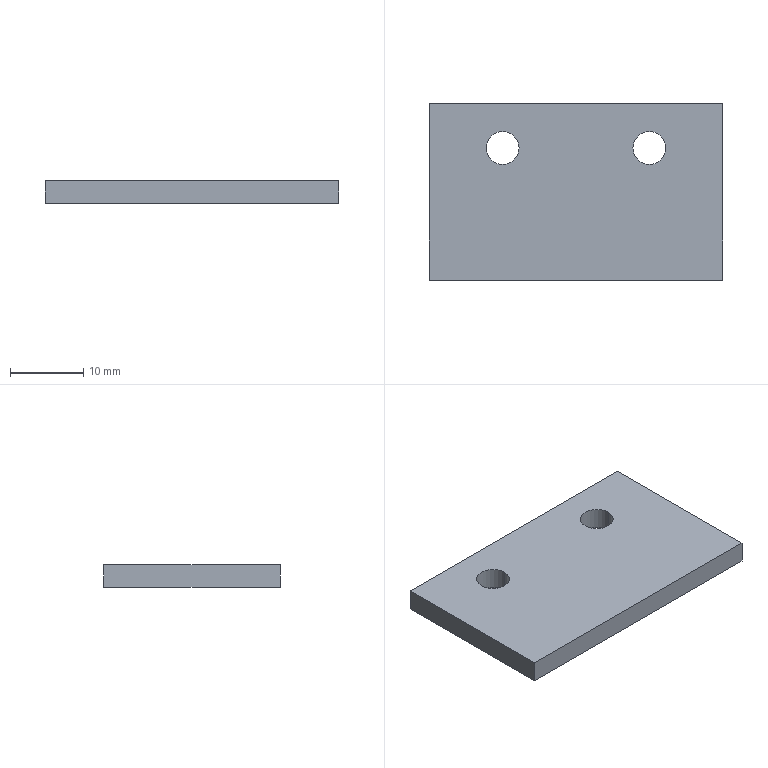Part | STEP file | Guide pressure plate | 1 solid | 10 faces | box 40 x 24 x 3 mm | volume 2785 mm3 | plane 6 | cylinder 4 | commonest cylinder face diameters 4.5 x4
STEP:
#1=CARTESIAN_POINT('',(7.75,6.,0.));
#2=VERTEX_POINT('',#1);
#3=CARTESIAN_POINT('',(12.25,6.,0.));
#4=VERTEX_POINT('',#3);
#5=CARTESIAN_POINT('',(10.,6.,0.));
#6=DIRECTION('',(0.,0.,1.));
#7=DIRECTION('',(1.,0.,0.));
#8=AXIS2_PLACEMENT_3D('',#5,#6,#7);
#9=CIRCLE('',#8,2.25);
#10=EDGE_CURVE('',#2,#4,#9,.T.);
#11=ORIENTED_EDGE('',*,*,#10,.F.);
#12=CARTESIAN_POINT('',(7.75,6.,3.));
#13=VERTEX_POINT('',#12);
#14=CARTESIAN_POINT('',(7.75,6.,0.));
#15=DIRECTION('',(0.,0.,1.));
#16=VECTOR('',#15,1000.);
#17=LINE('',#14,#16);
#18=EDGE_CURVE('',#2,#13,#17,.T.);
#19=ORIENTED_EDGE('',*,*,#18,.T.);
#20=CARTESIAN_POINT('',(12.25,6.,3.));
#21=VERTEX_POINT('',#20);
#22=CARTESIAN_POINT('',(10.,6.,3.));
#23=DIRECTION('',(0.,0.,1.));
#24=DIRECTION('',(1.,0.,0.));
#25=AXIS2_PLACEMENT_3D('',#22,#23,#24);
#26=CIRCLE('',#25,2.25);
#27=EDGE_CURVE('',#13,#21,#26,.T.);
#28=ORIENTED_EDGE('',*,*,#27,.T.);
#29=CARTESIAN_POINT('',(12.25,6.,0.));
#30=DIRECTION('',(0.,0.,1.));
#31=VECTOR('',#30,1000.);
#32=LINE('',#29,#31);
#33=EDGE_CURVE('',#4,#21,#32,.T.);
#34=ORIENTED_EDGE('',*,*,#33,.F.);
#35=EDGE_LOOP('',(#11,#19,#28,#34));
#36=FACE_OUTER_BOUND('',#35,.T.);
#37=CARTESIAN_POINT('',(10.,6.,0.));
#38=DIRECTION('',(0.,0.,1.));
#39=DIRECTION('',(1.,0.,0.));
#40=AXIS2_PLACEMENT_3D('',#37,#38,#39);
#41=CYLINDRICAL_SURFACE('',#40,2.25);
#42=ADVANCED_FACE('',(#36),#41,.F.);
#43=CARTESIAN_POINT('',(-12.25,6.,0.));
#44=VERTEX_POINT('',#43);
#45=CARTESIAN_POINT('',(-7.75,6.,0.));
#46=VERTEX_POINT('',#45);
#47=CARTESIAN_POINT('',(-10.,6.,0.));
#48=DIRECTION('',(0.,0.,1.));
#49=DIRECTION('',(1.,0.,0.));
#50=AXIS2_PLACEMENT_3D('',#47,#48,#49);
#51=CIRCLE('',#50,2.25);
#52=EDGE_CURVE('',#44,#46,#51,.T.);
#53=ORIENTED_EDGE('',*,*,#52,.F.);
#54=CARTESIAN_POINT('',(-12.25,6.,3.));
#55=VERTEX_POINT('',#54);
#56=CARTESIAN_POINT('',(-12.25,6.,0.));
#57=DIRECTION('',(0.,0.,1.));
#58=VECTOR('',#57,1000.);
#59=LINE('',#56,#58);
#60=EDGE_CURVE('',#44,#55,#59,.T.);
#61=ORIENTED_EDGE('',*,*,#60,.T.);
#62=CARTESIAN_POINT('',(-7.75,6.,3.));
#63=VERTEX_POINT('',#62);
#64=CARTESIAN_POINT('',(-10.,6.,3.));
#65=DIRECTION('',(0.,0.,1.));
#66=DIRECTION('',(1.,0.,0.));
#67=AXIS2_PLACEMENT_3D('',#64,#65,#66);
#68=CIRCLE('',#67,2.25);
#69=EDGE_CURVE('',#55,#63,#68,.T.);
#70=ORIENTED_EDGE('',*,*,#69,.T.);
#71=CARTESIAN_POINT('',(-7.75,6.,0.));
#72=DIRECTION('',(0.,0.,1.));
#73=VECTOR('',#72,1000.);
#74=LINE('',#71,#73);
#75=EDGE_CURVE('',#46,#63,#74,.T.);
#76=ORIENTED_EDGE('',*,*,#75,.F.);
#77=EDGE_LOOP('',(#53,#61,#70,#76));
#78=FACE_OUTER_BOUND('',#77,.T.);
#79=CARTESIAN_POINT('',(-10.,6.,0.));
#80=DIRECTION('',(0.,0.,1.));
#81=DIRECTION('',(1.,0.,0.));
#82=AXIS2_PLACEMENT_3D('',#79,#80,#81);
#83=CYLINDRICAL_SURFACE('',#82,2.25);
#84=ADVANCED_FACE('',(#78),#83,.F.);
#85=CARTESIAN_POINT('',(20.,-12.,0.));
#86=VERTEX_POINT('',#85);
#87=CARTESIAN_POINT('',(20.,12.,0.));
#88=VERTEX_POINT('',#87);
#89=CARTESIAN_POINT('',(20.,12.,0.));
#90=DIRECTION('',(0.,1.,0.));
#91=VECTOR('',#90,1000.);
#92=LINE('',#89,#91);
#93=EDGE_CURVE('',#86,#88,#92,.T.);
#94=ORIENTED_EDGE('',*,*,#93,.T.);
#95=CARTESIAN_POINT('',(20.,12.,3.));
#96=VERTEX_POINT('',#95);
#97=CARTESIAN_POINT('',(20.,12.,3.));
#98=DIRECTION('',(0.,0.,-1.));
#99=VECTOR('',#98,1000.);
#100=LINE('',#97,#99);
#101=EDGE_CURVE('',#96,#88,#100,.T.);
#102=ORIENTED_EDGE('',*,*,#101,.F.);
#103=CARTESIAN_POINT('',(20.,-12.,3.));
#104=VERTEX_POINT('',#103);
#105=CARTESIAN_POINT('',(20.,12.,3.));
#106=DIRECTION('',(0.,1.,0.));
#107=VECTOR('',#106,1000.);
#108=LINE('',#105,#107);
#109=EDGE_CURVE('',#104,#96,#108,.T.);
#110=ORIENTED_EDGE('',*,*,#109,.F.);
#111=CARTESIAN_POINT('',(20.,-12.,3.));
#112=DIRECTION('',(0.,0.,-1.));
#113=VECTOR('',#112,1000.);
#114=LINE('',#111,#113);
#115=EDGE_CURVE('',#104,#86,#114,.T.);
#116=ORIENTED_EDGE('',*,*,#115,.T.);
#117=EDGE_LOOP('',(#94,#102,#110,#116));
#118=FACE_OUTER_BOUND('',#117,.T.);
#119=CARTESIAN_POINT('',(20.,12.,3.));
#120=DIRECTION('',(-1.,0.,0.));
#121=DIRECTION('',(0.,-1.,0.));
#122=AXIS2_PLACEMENT_3D('',#119,#120,#121);
#123=PLANE('',#122);
#124=ADVANCED_FACE('',(#118),#123,.F.);
#125=CARTESIAN_POINT('',(-20.,12.,0.));
#126=VERTEX_POINT('',#125);
#127=CARTESIAN_POINT('',(-20.,12.,0.));
#128=DIRECTION('',(-1.,0.,0.));
#129=VECTOR('',#128,1000.);
#130=LINE('',#127,#129);
#131=EDGE_CURVE('',#88,#126,#130,.T.);
#132=ORIENTED_EDGE('',*,*,#131,.T.);
#133=CARTESIAN_POINT('',(-20.,12.,3.));
#134=VERTEX_POINT('',#133);
#135=CARTESIAN_POINT('',(-20.,12.,3.));
#136=DIRECTION('',(0.,0.,-1.));
#137=VECTOR('',#136,1000.);
#138=LINE('',#135,#137);
#139=EDGE_CURVE('',#134,#126,#138,.T.);
#140=ORIENTED_EDGE('',*,*,#139,.F.);
#141=CARTESIAN_POINT('',(-20.,12.,3.));
#142=DIRECTION('',(-1.,0.,0.));
#143=VECTOR('',#142,1000.);
#144=LINE('',#141,#143);
#145=EDGE_CURVE('',#96,#134,#144,.T.);
#146=ORIENTED_EDGE('',*,*,#145,.F.);
#147=ORIENTED_EDGE('',*,*,#101,.T.);
#148=EDGE_LOOP('',(#132,#140,#146,#147));
#149=FACE_OUTER_BOUND('',#148,.T.);
#150=CARTESIAN_POINT('',(-20.,12.,3.));
#151=DIRECTION('',(0.,-1.,0.));
#152=DIRECTION('',(0.,0.,-1.));
#153=AXIS2_PLACEMENT_3D('',#150,#151,#152);
#154=PLANE('',#153);
#155=ADVANCED_FACE('',(#149),#154,.F.);
#156=CARTESIAN_POINT('',(-20.,-12.,0.));
#157=VERTEX_POINT('',#156);
#158=CARTESIAN_POINT('',(-20.,12.,0.));
#159=DIRECTION('',(0.,-1.,0.));
#160=VECTOR('',#159,1000.);
#161=LINE('',#158,#160);
#162=EDGE_CURVE('',#126,#157,#161,.T.);
#163=ORIENTED_EDGE('',*,*,#162,.T.);
#164=CARTESIAN_POINT('',(-20.,-12.,3.));
#165=VERTEX_POINT('',#164);
#166=CARTESIAN_POINT('',(-20.,-12.,3.));
#167=DIRECTION('',(0.,0.,-1.));
#168=VECTOR('',#167,1000.);
#169=LINE('',#166,#168);
#170=EDGE_CURVE('',#165,#157,#169,.T.);
#171=ORIENTED_EDGE('',*,*,#170,.F.);
#172=CARTESIAN_POINT('',(-20.,12.,3.));
#173=DIRECTION('',(0.,-1.,0.));
#174=VECTOR('',#173,1000.);
#175=LINE('',#172,#174);
#176=EDGE_CURVE('',#134,#165,#175,.T.);
#177=ORIENTED_EDGE('',*,*,#176,.F.);
#178=ORIENTED_EDGE('',*,*,#139,.T.);
#179=EDGE_LOOP('',(#163,#171,#177,#178));
#180=FACE_OUTER_BOUND('',#179,.T.);
#181=CARTESIAN_POINT('',(-20.,12.,3.));
#182=DIRECTION('',(1.,0.,0.));
#183=DIRECTION('',(0.,1.,0.));
#184=AXIS2_PLACEMENT_3D('',#181,#182,#183);
#185=PLANE('',#184);
#186=ADVANCED_FACE('',(#180),#185,.F.);
#187=CARTESIAN_POINT('',(-20.,-12.,0.));
#188=DIRECTION('',(1.,0.,0.));
#189=VECTOR('',#188,1000.);
#190=LINE('',#187,#189);
#191=EDGE_CURVE('',#157,#86,#190,.T.);
#192=ORIENTED_EDGE('',*,*,#191,.T.);
#193=ORIENTED_EDGE('',*,*,#115,.F.);
#194=CARTESIAN_POINT('',(-20.,-12.,3.));
#195=DIRECTION('',(1.,0.,0.));
#196=VECTOR('',#195,1000.);
#197=LINE('',#194,#196);
#198=EDGE_CURVE('',#165,#104,#197,.T.);
#199=ORIENTED_EDGE('',*,*,#198,.F.);
#200=ORIENTED_EDGE('',*,*,#170,.T.);
#201=EDGE_LOOP('',(#192,#193,#199,#200));
#202=FACE_OUTER_BOUND('',#201,.T.);
#203=CARTESIAN_POINT('',(-20.,-12.,3.));
#204=DIRECTION('',(0.,1.,0.));
#205=DIRECTION('',(0.,0.,1.));
#206=AXIS2_PLACEMENT_3D('',#203,#204,#205);
#207=PLANE('',#206);
#208=ADVANCED_FACE('',(#202),#207,.F.);
#209=CARTESIAN_POINT('',(10.,6.,3.));
#210=DIRECTION('',(0.,0.,1.));
#211=DIRECTION('',(1.,0.,0.));
#212=AXIS2_PLACEMENT_3D('',#209,#210,#211);
#213=CIRCLE('',#212,2.25);
#214=EDGE_CURVE('',#21,#13,#213,.T.);
#215=ORIENTED_EDGE('',*,*,#214,.F.);
#216=ORIENTED_EDGE('',*,*,#27,.F.);
#217=EDGE_LOOP('',(#215,#216));
#218=FACE_BOUND('',#217,.T.);
#219=CARTESIAN_POINT('',(-10.,6.,3.));
#220=DIRECTION('',(0.,0.,1.));
#221=DIRECTION('',(1.,0.,0.));
#222=AXIS2_PLACEMENT_3D('',#219,#220,#221);
#223=CIRCLE('',#222,2.25);
#224=EDGE_CURVE('',#63,#55,#223,.T.);
#225=ORIENTED_EDGE('',*,*,#224,.F.);
#226=ORIENTED_EDGE('',*,*,#69,.F.);
#227=EDGE_LOOP('',(#225,#226));
#228=FACE_BOUND('',#227,.T.);
#229=ORIENTED_EDGE('',*,*,#109,.T.);
#230=ORIENTED_EDGE('',*,*,#145,.T.);
#231=ORIENTED_EDGE('',*,*,#176,.T.);
#232=ORIENTED_EDGE('',*,*,#198,.T.);
#233=EDGE_LOOP('',(#229,#230,#231,#232));
#234=FACE_OUTER_BOUND('',#233,.T.);
#235=CARTESIAN_POINT('',(0.,0.,3.));
#236=DIRECTION('',(0.,0.,1.));
#237=DIRECTION('',(1.,0.,0.));
#238=AXIS2_PLACEMENT_3D('',#235,#236,#237);
#239=PLANE('',#238);
#240=ADVANCED_FACE('',(#218,#228,#234),#239,.T.);
#241=CARTESIAN_POINT('',(10.,6.,0.));
#242=DIRECTION('',(0.,0.,1.));
#243=DIRECTION('',(1.,0.,0.));
#244=AXIS2_PLACEMENT_3D('',#241,#242,#243);
#245=CIRCLE('',#244,2.25);
#246=EDGE_CURVE('',#4,#2,#245,.T.);
#247=ORIENTED_EDGE('',*,*,#246,.T.);
#248=ORIENTED_EDGE('',*,*,#10,.T.);
#249=EDGE_LOOP('',(#247,#248));
#250=FACE_BOUND('',#249,.T.);
#251=CARTESIAN_POINT('',(-10.,6.,0.));
#252=DIRECTION('',(0.,0.,1.));
#253=DIRECTION('',(1.,0.,0.));
#254=AXIS2_PLACEMENT_3D('',#251,#252,#253);
#255=CIRCLE('',#254,2.25);
#256=EDGE_CURVE('',#46,#44,#255,.T.);
#257=ORIENTED_EDGE('',*,*,#256,.T.);
#258=ORIENTED_EDGE('',*,*,#52,.T.);
#259=EDGE_LOOP('',(#257,#258));
#260=FACE_BOUND('',#259,.T.);
#261=ORIENTED_EDGE('',*,*,#93,.F.);
#262=ORIENTED_EDGE('',*,*,#191,.F.);
#263=ORIENTED_EDGE('',*,*,#162,.F.);
#264=ORIENTED_EDGE('',*,*,#131,.F.);
#265=EDGE_LOOP('',(#261,#262,#263,#264));
#266=FACE_OUTER_BOUND('',#265,.T.);
#267=CARTESIAN_POINT('',(0.,0.,0.));
#268=DIRECTION('',(0.,0.,1.));
#269=DIRECTION('',(1.,0.,0.));
#270=AXIS2_PLACEMENT_3D('',#267,#268,#269);
#271=PLANE('',#270);
#272=ADVANCED_FACE('',(#250,#260,#266),#271,.F.);
#273=ORIENTED_EDGE('',*,*,#60,.F.);
#274=ORIENTED_EDGE('',*,*,#256,.F.);
#275=ORIENTED_EDGE('',*,*,#75,.T.);
#276=ORIENTED_EDGE('',*,*,#224,.T.);
#277=EDGE_LOOP('',(#273,#274,#275,#276));
#278=FACE_OUTER_BOUND('',#277,.T.);
#279=CARTESIAN_POINT('',(-10.,6.,0.));
#280=DIRECTION('',(0.,0.,1.));
#281=DIRECTION('',(1.,0.,0.));
#282=AXIS2_PLACEMENT_3D('',#279,#280,#281);
#283=CYLINDRICAL_SURFACE('',#282,2.25);
#284=ADVANCED_FACE('',(#278),#283,.F.);
#285=ORIENTED_EDGE('',*,*,#18,.F.);
#286=ORIENTED_EDGE('',*,*,#246,.F.);
#287=ORIENTED_EDGE('',*,*,#33,.T.);
#288=ORIENTED_EDGE('',*,*,#214,.T.);
#289=EDGE_LOOP('',(#285,#286,#287,#288));
#290=FACE_OUTER_BOUND('',#289,.T.);
#291=CARTESIAN_POINT('',(10.,6.,0.));
#292=DIRECTION('',(0.,0.,1.));
#293=DIRECTION('',(1.,0.,0.));
#294=AXIS2_PLACEMENT_3D('',#291,#292,#293);
#295=CYLINDRICAL_SURFACE('',#294,2.25);
#296=ADVANCED_FACE('',(#290),#295,.F.);
#297=CLOSED_SHELL('',(#42,#84,#124,#155,#186,#208,#240,#272,#284,#296));
#298=MANIFOLD_SOLID_BREP('',#297);
#299=CARTESIAN_POINT('',(0.,0.,0.));
#300=DIRECTION('',(0.,0.,1.));
#301=DIRECTION('',(1.,0.,0.));
#302=AXIS2_PLACEMENT_3D('',#299,#300,#301);
#303=(LENGTH_UNIT()NAMED_UNIT(*)SI_UNIT(.MILLI.,.METRE.));
#304=UNCERTAINTY_MEASURE_WITH_UNIT(LENGTH_MEASURE(0.00001),#303,'','');
#305=(NAMED_UNIT(*)PLANE_ANGLE_UNIT()SI_UNIT($,.RADIAN.));
#306=(NAMED_UNIT(*)SI_UNIT($,.STERADIAN.)SOLID_ANGLE_UNIT());
#307=(GEOMETRIC_REPRESENTATION_CONTEXT(3)GLOBAL_UNCERTAINTY_ASSIGNED_CONTEXT((#304))GLOBAL_UNIT_ASSIGNED_CONTEXT((#303,#305,#306))REPRESENTATION_CONTEXT('',''));
#308=ADVANCED_BREP_SHAPE_REPRESENTATION('',(#298,#302),#307);